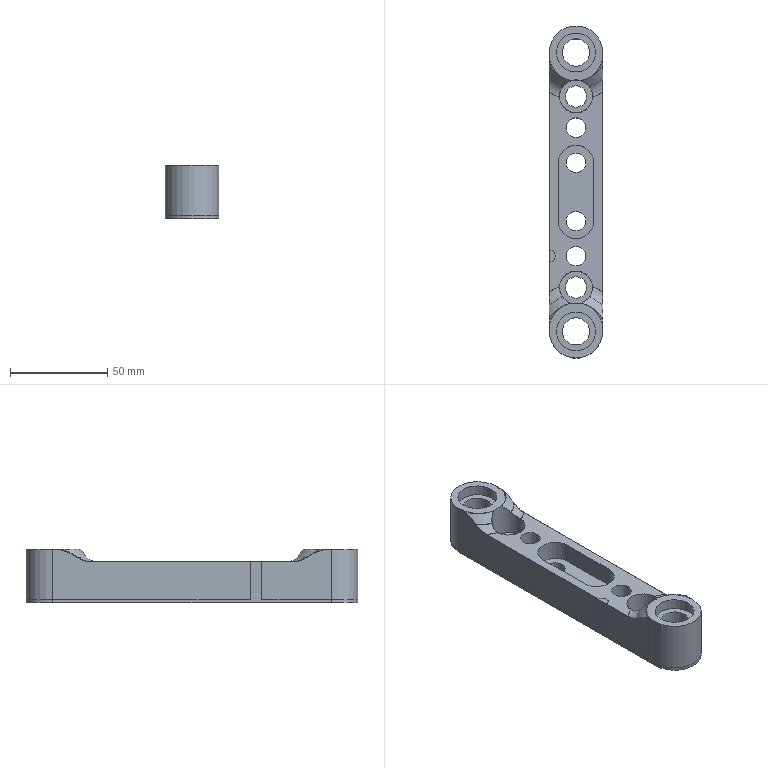NC program | NX | posted with a generic post | part box 27.4 x 170.48 x 27.5 mm
Lines 14728 to 16455 of 16455:
(DRILLING_1 , TOOL : D14钻头)
N29376 T12 M6
N29378 G54
N29380 G17 G0 G90 X-71.54 Y0. B0. C0. S800 M3
N29382 G43 Z30. H12
N29384 G94 G81 G98 Z-28.5 F100. R3.
N29386 X71.54
N29388 G80
N29390 G0 X71.54 Y0. Z30.
N29392 M5
(DRILLING_2 , TOOL : D10镗刀)
N29394 T13 M6
N29396 G54
N29398 G17 G0 G90 X-33. Y0. B0. C0. S800 M3
N29400 G43 Z30. H13
N29402 G94 G86 G98 Z-29.5 F60. R-3.5
N29404 X33.
N29406 G80
N29408 G0 X33. Y0. Z30.
N29410 M5
(DRILLING_3 , TOOL : D20镗刀)
N29412 T14 M6
N29414 G54
N29416 G17 G0 G90 X-71.54 Y0. B0. C0. S800 M3
N29418 G43 Z30. H14
N29420 G94 G86 G98 Z-5.5 F60. R3.
N29422 X71.54
N29424 G80
N29426 G0 X71.54 Y0. Z30.
N29428 M5
(PLANAR_MILL_3_COPY_COPY_COPY_1_COPY , TOOL : D6倒角刀)
N29430 T11 M6
N29432 G54
N29434 G17 G0 G90 X-69.54 Y3.231 B0. C0. S3500 M3
N29436 G43 Z30. H11
N29438 Z-5.8
N29440 G94 G1 Z-7.8 F800.
N29442 Y3.8
N29444 G3 X-71.54 Y5.8 R2.
N29446 X-77.34 Y0. R5.8
N29448 X-71.54 Y5.8 R-5.8
N29450 X-73.54 Y3.8 R2.
N29452 G1 Y3.231
N29454 Z-5.8
N29456 G0 Z30.
N29458 X73.54
N29460 Z-5.8
N29462 G1 Z-7.8
N29464 Y3.8
N29466 G3 X71.54 Y5.8 R2.
N29468 X65.74 Y0. R5.8
N29470 X71.54 Y5.8 R-5.8
N29472 X69.54 Y3.8 R2.
N29474 G1 Y3.231
N29476 Z-5.8
N29478 G0 Z30.
(PLANAR_MILL_3_COPY_COPY_COPY_1_COPY_COPY_1 , TOOL : D6倒角刀)
N29480 X-14. Y1.96
N29482 Z-16.5
N29484 G1 Z-18.5
N29486 Y2.2
N29488 G3 X-15. Y3.2 R1.
N29490 X-18.2 Y0. R3.2
N29492 X-15. Y3.2 R-3.2
N29494 X-16. Y2.2 R1.
N29496 G1 Y1.96
N29498 Z-16.5
N29500 G0 Z30.
N29502 X16.
N29504 Z-16.5
N29506 G1 Z-18.5
N29508 Y2.2
N29510 G3 X15. Y3.2 R1.
N29512 X11.8 Y0. R3.2
N29514 X15. Y3.2 R-3.2
N29516 X14. Y2.2 R1.
N29518 G1 Y1.96
N29520 Z-16.5
N29522 G0 Z30.
N29524 M5
(THREAD_MILLING , TOOL : M16螺纹铣刀)
N29526 T15 M6
N29528 G54
N29530 G17 G0 G90 X-71.54 Y0. B0. C0. S3000 M3
N29532 G43 Z30. H15
N29534 Z-29.182
N29536 G41 G94 G1 X-72.223 Y-1.391 F300. D15
N29538 G3 X-71.54 Y-2.3 Z-29. R0.711
N29540 X-71.54 Y-2.3 Z-27. I0. J2.3
N29542 X-70.857 Y-1.391 Z-26.818 R0.711
N29544 G40
N29546 G1 X-71.54 Y0.
N29548 G0 Z-23.182
N29550 G41 G1 X-72.223 Y-1.391
N29552 G3 X-71.54 Y-2.3 Z-23. R0.711
N29554 X-71.54 Y-2.3 Z-21. I0. J2.3
N29556 X-70.857 Y-1.391 Z-20.818 R0.711
N29558 G40
N29560 G1 X-71.54 Y0.
N29562 G0 Z-17.182
N29564 G41 G1 X-72.223 Y-1.391
N29566 G3 X-71.54 Y-2.3 Z-17. R0.711
N29568 X-71.54 Y-2.3 Z-15. I0. J2.3
N29570 X-70.857 Y-1.391 Z-14.818 R0.711
N29572 G40
N29574 G1 X-71.54 Y0.
N29576 G0 Z-11.182
N29578 G41 G1 X-72.223 Y-1.391
N29580 G3 X-71.54 Y-2.3 Z-11. R0.711
N29582 X-71.54 Y-2.3 Z-9. I0. J2.3
N29584 X-70.857 Y-1.391 Z-8.818 R0.711
N29586 G40
N29588 G1 X-71.54 Y0.
N29590 G0 Z-5.182
N29592 G41 G1 X-72.223 Y-1.391
N29594 G3 X-71.54 Y-2.3 Z-5. R0.711
N29596 X-71.54 Y-2.3 Z-3. I0. J2.3
N29598 X-71.54 Y-2.3 Z-1. I0. J2.3
N29600 X-70.857 Y-1.391 Z-0.818 R0.711
N29602 G40
N29604 G1 X-71.54 Y0.
N29606 G0 Z-29.22
N29608 G41 G1 X-72.371 Y-1.308
N29610 G3 X-71.54 Y-2.55 Z-29. R0.899
N29612 X-71.54 Y-2.55 Z-27. I0. J2.55
N29614 X-70.709 Y-1.308 Z-26.78 R0.899
N29616 G40
N29618 G1 X-71.54 Y0.
N29620 G0 Z-23.22
N29622 G41 G1 X-72.371 Y-1.308
N29624 G3 X-71.54 Y-2.55 Z-23. R0.899
N29626 X-71.54 Y-2.55 Z-21. I0. J2.55
N29628 X-70.709 Y-1.308 Z-20.78 R0.899
N29630 G40
N29632 G1 X-71.54 Y0.
N29634 G0 Z-17.22
N29636 G41 G1 X-72.371 Y-1.308
N29638 G3 X-71.54 Y-2.55 Z-17. R0.899
N29640 X-71.54 Y-2.55 Z-15. I0. J2.55
N29642 X-70.709 Y-1.308 Z-14.78 R0.899
N29644 G40
N29646 G1 X-71.54 Y0.
N29648 G0 Z-11.22
N29650 G41 G1 X-72.371 Y-1.308
N29652 G3 X-71.54 Y-2.55 Z-11. R0.899
N29654 X-71.54 Y-2.55 Z-9. I0. J2.55
N29656 X-70.709 Y-1.308 Z-8.78 R0.899
N29658 G40
N29660 G1 X-71.54 Y0.
N29662 G0 Z-5.22
N29664 G41 G1 X-72.371 Y-1.308
N29666 G3 X-71.54 Y-2.55 Z-5. R0.899
N29668 X-71.54 Y-2.55 Z-3. I0. J2.55
N29670 X-71.54 Y-2.55 Z-1. I0. J2.55
N29672 X-70.709 Y-1.308 Z-0.78 R0.899
N29674 G40
N29676 G1 X-71.54 Y0.
N29678 G0 Z-29.251
N29680 G41 G1 X-72.49 Y-1.225
N29682 G3 X-71.54 Y-2.8 Z-29. R1.074
N29684 X-71.54 Y-2.8 Z-27. I0. J2.8
N29686 X-70.59 Y-1.225 Z-26.749 R1.074
N29688 G40
N29690 G1 X-71.54 Y0.
N29692 G0 Z-23.251
N29694 G41 G1 X-72.49 Y-1.225
N29696 G3 X-71.54 Y-2.8 Z-23. R1.074
N29698 X-71.54 Y-2.8 Z-21. I0. J2.8
N29700 X-70.59 Y-1.225 Z-20.749 R1.074
N29702 G40
N29704 G1 X-71.54 Y0.
N29706 G0 Z-17.251
N29708 G41 G1 X-72.49 Y-1.225
N29710 G3 X-71.54 Y-2.8 Z-17. R1.074
N29712 X-71.54 Y-2.8 Z-15. I0. J2.8
N29714 X-70.59 Y-1.225 Z-14.749 R1.074
N29716 G40
N29718 G1 X-71.54 Y0.
N29720 G0 Z-11.251
N29722 G41 G1 X-72.49 Y-1.225
N29724 G3 X-71.54 Y-2.8 Z-11. R1.074
N29726 X-71.54 Y-2.8 Z-9. I0. J2.8
N29728 X-70.59 Y-1.225 Z-8.749 R1.074
N29730 G40
N29732 G1 X-71.54 Y0.
N29734 G0 Z-5.251
N29736 G41 G1 X-72.49 Y-1.225
N29738 G3 X-71.54 Y-2.8 Z-5. R1.074
N29740 X-71.54 Y-2.8 Z-3. I0. J2.8
N29742 X-71.54 Y-2.8 Z-1. I0. J2.8
N29744 X-70.59 Y-1.225 Z-0.749 R1.074
N29746 G40
N29748 G1 X-71.54 Y0.
N29750 G0 Z-29.277
N29752 G41 G1 X-72.587 Y-1.143
N29754 G3 X-71.54 Y-3.05 Z-29. R1.241
N29756 X-71.54 Y-3.05 Z-27. I0. J3.05
N29758 X-70.493 Y-1.143 Z-26.723 R1.241
N29760 G40
N29762 G1 X-71.54 Y0.
N29764 G0 Z-23.277
N29766 G41 G1 X-72.587 Y-1.143
N29768 G3 X-71.54 Y-3.05 Z-23. R1.241
N29770 X-71.54 Y-3.05 Z-21. I0. J3.05
N29772 X-70.493 Y-1.143 Z-20.723 R1.241
N29774 G40
N29776 G1 X-71.54 Y0.
N29778 G0 Z-17.277
N29780 G41 G1 X-72.587 Y-1.143
N29782 G3 X-71.54 Y-3.05 Z-17. R1.241
N29784 X-71.54 Y-3.05 Z-15. I0. J3.05
N29786 X-70.493 Y-1.143 Z-14.723 R1.241
N29788 G40
N29790 G1 X-71.54 Y0.
N29792 G0 Z-11.277
N29794 G41 G1 X-72.587 Y-1.143
N29796 G3 X-71.54 Y-3.05 Z-11. R1.241
N29798 X-71.54 Y-3.05 Z-9. I0. J3.05
N29800 X-70.493 Y-1.143 Z-8.723 R1.241
N29802 G40
N29804 G1 X-71.54 Y0.
N29806 G0 Z-5.277
N29808 G41 G1 X-72.587 Y-1.143
N29810 G3 X-71.54 Y-3.05 Z-5. R1.241
N29812 X-71.54 Y-3.05 Z-3. I0. J3.05
N29814 X-71.54 Y-3.05 Z-1. I0. J3.05
N29816 X-70.493 Y-1.143 Z-0.723 R1.241
N29818 G40
N29820 G1 X-71.54 Y0.
N29822 G0 Z-29.277
N29824 G41 G1 X-72.587 Y-1.143
N29826 G3 X-71.54 Y-3.05 Z-29. R1.241
N29828 X-71.54 Y-3.05 Z-27. I0. J3.05
N29830 X-70.493 Y-1.143 Z-26.723 R1.241
N29832 G40
N29834 G1 X-71.54 Y0.
N29836 G0 Z-23.277
N29838 G41 G1 X-72.587 Y-1.143
N29840 G3 X-71.54 Y-3.05 Z-23. R1.241
N29842 X-71.54 Y-3.05 Z-21. I0. J3.05
N29844 X-70.493 Y-1.143 Z-20.723 R1.241
N29846 G40
N29848 G1 X-71.54 Y0.
N29850 G0 Z-17.277
N29852 G41 G1 X-72.587 Y-1.143
N29854 G3 X-71.54 Y-3.05 Z-17. R1.241
N29856 X-71.54 Y-3.05 Z-15. I0. J3.05
N29858 X-70.493 Y-1.143 Z-14.723 R1.241
N29860 G40
N29862 G1 X-71.54 Y0.
N29864 G0 Z-11.277
N29866 G41 G1 X-72.587 Y-1.143
N29868 G3 X-71.54 Y-3.05 Z-11. R1.241
N29870 X-71.54 Y-3.05 Z-9. I0. J3.05
N29872 X-70.493 Y-1.143 Z-8.723 R1.241
N29874 G40
N29876 G1 X-71.54 Y0.
N29878 G0 Z-5.277
N29880 G41 G1 X-72.587 Y-1.143
N29882 G3 X-71.54 Y-3.05 Z-5. R1.241
N29884 X-71.54 Y-3.05 Z-3. I0. J3.05
N29886 X-71.54 Y-3.05 Z-1. I0. J3.05
N29888 X-70.493 Y-1.143 Z-0.723 R1.241
N29890 G40
N29892 G1 X-71.54 Y0.
N29894 G0 Z-29.277
N29896 G41 G1 X-72.587 Y-1.143
N29898 G3 X-71.54 Y-3.05 Z-29. R1.241
N29900 X-71.54 Y-3.05 Z-27. I0. J3.05
N29902 X-70.493 Y-1.143 Z-26.723 R1.241
N29904 G40
N29906 G1 X-71.54 Y0.
N29908 G0 Z-23.277
N29910 G41 G1 X-72.587 Y-1.143
N29912 G3 X-71.54 Y-3.05 Z-23. R1.241
N29914 X-71.54 Y-3.05 Z-21. I0. J3.05
N29916 X-70.493 Y-1.143 Z-20.723 R1.241
N29918 G40
N29920 G1 X-71.54 Y0.
N29922 G0 Z-17.277
N29924 G41 G1 X-72.587 Y-1.143
N29926 G3 X-71.54 Y-3.05 Z-17. R1.241
N29928 X-71.54 Y-3.05 Z-15. I0. J3.05
N29930 X-70.493 Y-1.143 Z-14.723 R1.241
N29932 G40
N29934 G1 X-71.54 Y0.
N29936 G0 Z-11.277
N29938 G41 G1 X-72.587 Y-1.143
N29940 G3 X-71.54 Y-3.05 Z-11. R1.241
N29942 X-71.54 Y-3.05 Z-9. I0. J3.05
N29944 X-70.493 Y-1.143 Z-8.723 R1.241
N29946 G40
N29948 G1 X-71.54 Y0.
N29950 G0 Z-5.277
N29952 G41 G1 X-72.587 Y-1.143
N29954 G3 X-71.54 Y-3.05 Z-5. R1.241
N29956 X-71.54 Y-3.05 Z-3. I0. J3.05
N29958 X-71.54 Y-3.05 Z-1. I0. J3.05
N29960 X-70.493 Y-1.143 Z-0.723 R1.241
N29962 G40
N29964 G1 X-71.54 Y0.
N29966 G0 Z30.
N29968 X71.54
N29970 Z-29.182
N29972 G41 G1 X70.857 Y-1.391
N29974 G3 X71.54 Y-2.3 Z-29. R0.711
N29976 X71.54 Y-2.3 Z-27. I0. J2.3
N29978 X72.223 Y-1.391 Z-26.818 R0.711
N29980 G40
N29982 G1 X71.54 Y0.
N29984 G0 Z-23.182
N29986 G41 G1 X70.857 Y-1.391
N29988 G3 X71.54 Y-2.3 Z-23. R0.711
N29990 X71.54 Y-2.3 Z-21. I0. J2.3
N29992 X72.223 Y-1.391 Z-20.818 R0.711
N29994 G40
N29996 G1 X71.54 Y0.
N29998 G0 Z-17.182
N30000 G41 G1 X70.857 Y-1.391
N30002 G3 X71.54 Y-2.3 Z-17. R0.711
N30004 X71.54 Y-2.3 Z-15. I0. J2.3
N30006 X72.223 Y-1.391 Z-14.818 R0.711
N30008 G40
N30010 G1 X71.54 Y0.
N30012 G0 Z-11.182
N30014 G41 G1 X70.857 Y-1.391
N30016 G3 X71.54 Y-2.3 Z-11. R0.711
N30018 X71.54 Y-2.3 Z-9. I0. J2.3
N30020 X72.223 Y-1.391 Z-8.818 R0.711
N30022 G40
N30024 G1 X71.54 Y0.
N30026 G0 Z-5.182
N30028 G41 G1 X70.857 Y-1.391
N30030 G3 X71.54 Y-2.3 Z-5. R0.711
N30032 X71.54 Y-2.3 Z-3. I0. J2.3
N30034 X71.54 Y-2.3 Z-1. I0. J2.3
N30036 X72.223 Y-1.391 Z-0.818 R0.711
N30038 G40
N30040 G1 X71.54 Y0.
N30042 G0 Z-29.22
N30044 G41 G1 X70.709 Y-1.308
N30046 G3 X71.54 Y-2.55 Z-29. R0.899
N30048 X71.54 Y-2.55 Z-27. I0. J2.55
N30050 X72.371 Y-1.308 Z-26.78 R0.899
N30052 G40
N30054 G1 X71.54 Y0.
N30056 G0 Z-23.22
N30058 G41 G1 X70.709 Y-1.308
N30060 G3 X71.54 Y-2.55 Z-23. R0.899
N30062 X71.54 Y-2.55 Z-21. I0. J2.55
N30064 X72.371 Y-1.308 Z-20.78 R0.899
N30066 G40
N30068 G1 X71.54 Y0.
N30070 G0 Z-17.22
N30072 G41 G1 X70.709 Y-1.308
N30074 G3 X71.54 Y-2.55 Z-17. R0.899
N30076 X71.54 Y-2.55 Z-15. I0. J2.55
N30078 X72.371 Y-1.308 Z-14.78 R0.899
N30080 G40
N30082 G1 X71.54 Y0.
N30084 G0 Z-11.22
N30086 G41 G1 X70.709 Y-1.308
N30088 G3 X71.54 Y-2.55 Z-11. R0.899
N30090 X71.54 Y-2.55 Z-9. I0. J2.55
N30092 X72.371 Y-1.308 Z-8.78 R0.899
N30094 G40
N30096 G1 X71.54 Y0.
N30098 G0 Z-5.22
N30100 G41 G1 X70.709 Y-1.308
N30102 G3 X71.54 Y-2.55 Z-5. R0.899
N30104 X71.54 Y-2.55 Z-3. I0. J2.55
N30106 X71.54 Y-2.55 Z-1. I0. J2.55
N30108 X72.371 Y-1.308 Z-0.78 R0.899
N30110 G40
N30112 G1 X71.54 Y0.
N30114 G0 Z-29.251
N30116 G41 G1 X70.59 Y-1.225
N30118 G3 X71.54 Y-2.8 Z-29. R1.074
N30120 X71.54 Y-2.8 Z-27. I0. J2.8
N30122 X72.49 Y-1.225 Z-26.749 R1.074
N30124 G40
N30126 G1 X71.54 Y0.
N30128 G0 Z-23.251
N30130 G41 G1 X70.59 Y-1.225
N30132 G3 X71.54 Y-2.8 Z-23. R1.074
N30134 X71.54 Y-2.8 Z-21. I0. J2.8
N30136 X72.49 Y-1.225 Z-20.749 R1.074
N30138 G40
N30140 G1 X71.54 Y0.
N30142 G0 Z-17.251
N30144 G41 G1 X70.59 Y-1.225
N30146 G3 X71.54 Y-2.8 Z-17. R1.074
N30148 X71.54 Y-2.8 Z-15. I0. J2.8
N30150 X72.49 Y-1.225 Z-14.749 R1.074
N30152 G40
N30154 G1 X71.54 Y0.
N30156 G0 Z-11.251
N30158 G41 G1 X70.59 Y-1.225
N30160 G3 X71.54 Y-2.8 Z-11. R1.074
N30162 X71.54 Y-2.8 Z-9. I0. J2.8
N30164 X72.49 Y-1.225 Z-8.749 R1.074
N30166 G40
N30168 G1 X71.54 Y0.
N30170 G0 Z-5.251
N30172 G41 G1 X70.59 Y-1.225
N30174 G3 X71.54 Y-2.8 Z-5. R1.074
N30176 X71.54 Y-2.8 Z-3. I0. J2.8
N30178 X71.54 Y-2.8 Z-1. I0. J2.8
N30180 X72.49 Y-1.225 Z-0.749 R1.074
N30182 G40
N30184 G1 X71.54 Y0.
N30186 G0 Z-29.277
N30188 G41 G1 X70.493 Y-1.143
N30190 G3 X71.54 Y-3.05 Z-29. R1.241
N30192 X71.54 Y-3.05 Z-27. I0. J3.05
N30194 X72.587 Y-1.143 Z-26.723 R1.241
N30196 G40
N30198 G1 X71.54 Y0.
N30200 G0 Z-23.277
N30202 G41 G1 X70.493 Y-1.143
N30204 G3 X71.54 Y-3.05 Z-23. R1.241
N30206 X71.54 Y-3.05 Z-21. I0. J3.05
N30208 X72.587 Y-1.143 Z-20.723 R1.241
N30210 G40
N30212 G1 X71.54 Y0.
N30214 G0 Z-17.277
N30216 G41 G1 X70.493 Y-1.143
N30218 G3 X71.54 Y-3.05 Z-17. R1.241
N30220 X71.54 Y-3.05 Z-15. I0. J3.05
N30222 X72.587 Y-1.143 Z-14.723 R1.241
N30224 G40
N30226 G1 X71.54 Y0.
N30228 G0 Z-11.277
N30230 G41 G1 X70.493 Y-1.143
N30232 G3 X71.54 Y-3.05 Z-11. R1.241
N30234 X71.54 Y-3.05 Z-9. I0. J3.05
N30236 X72.587 Y-1.143 Z-8.723 R1.241
N30238 G40
N30240 G1 X71.54 Y0.
N30242 G0 Z-5.277
N30244 G41 G1 X70.493 Y-1.143
N30246 G3 X71.54 Y-3.05 Z-5. R1.241
N30248 X71.54 Y-3.05 Z-3. I0. J3.05
N30250 X71.54 Y-3.05 Z-1. I0. J3.05
N30252 X72.587 Y-1.143 Z-0.723 R1.241
N30254 G40
N30256 G1 X71.54 Y0.
N30258 G0 Z-29.277
N30260 G41 G1 X70.493 Y-1.143
N30262 G3 X71.54 Y-3.05 Z-29. R1.241
N30264 X71.54 Y-3.05 Z-27. I0. J3.05
N30266 X72.587 Y-1.143 Z-26.723 R1.241
N30268 G40
N30270 G1 X71.54 Y0.
N30272 G0 Z-23.277
N30274 G41 G1 X70.493 Y-1.143
N30276 G3 X71.54 Y-3.05 Z-23. R1.241
N30278 X71.54 Y-3.05 Z-21. I0. J3.05
N30280 X72.587 Y-1.143 Z-20.723 R1.241
N30282 G40
N30284 G1 X71.54 Y0.
N30286 G0 Z-17.277
N30288 G41 G1 X70.493 Y-1.143
N30290 G3 X71.54 Y-3.05 Z-17. R1.241
N30292 X71.54 Y-3.05 Z-15. I0. J3.05
N30294 X72.587 Y-1.143 Z-14.723 R1.241
N30296 G40
N30298 G1 X71.54 Y0.
N30300 G0 Z-11.277
N30302 G41 G1 X70.493 Y-1.143
N30304 G3 X71.54 Y-3.05 Z-11. R1.241
N30306 X71.54 Y-3.05 Z-9. I0. J3.05
N30308 X72.587 Y-1.143 Z-8.723 R1.241
N30310 G40
N30312 G1 X71.54 Y0.
N30314 G0 Z-5.277
N30316 G41 G1 X70.493 Y-1.143
N30318 G3 X71.54 Y-3.05 Z-5. R1.241
N30320 X71.54 Y-3.05 Z-3. I0. J3.05
N30322 X71.54 Y-3.05 Z-1. I0. J3.05
N30324 X72.587 Y-1.143 Z-0.723 R1.241
N30326 G40
N30328 G1 X71.54 Y0.
N30330 G0 Z-29.277
N30332 G41 G1 X70.493 Y-1.143
N30334 G3 X71.54 Y-3.05 Z-29. R1.241
N30336 X71.54 Y-3.05 Z-27. I0. J3.05
N30338 X72.587 Y-1.143 Z-26.723 R1.241
N30340 G40
N30342 G1 X71.54 Y0.
N30344 G0 Z-23.277
N30346 G41 G1 X70.493 Y-1.143
N30348 G3 X71.54 Y-3.05 Z-23. R1.241
N30350 X71.54 Y-3.05 Z-21. I0. J3.05
N30352 X72.587 Y-1.143 Z-20.723 R1.241
N30354 G40
N30356 G1 X71.54 Y0.
N30358 G0 Z-17.277
N30360 G41 G1 X70.493 Y-1.143
N30362 G3 X71.54 Y-3.05 Z-17. R1.241
N30364 X71.54 Y-3.05 Z-15. I0. J3.05
N30366 X72.587 Y-1.143 Z-14.723 R1.241
N30368 G40
N30370 G1 X71.54 Y0.
N30372 G0 Z-11.277
N30374 G41 G1 X70.493 Y-1.143
N30376 G3 X71.54 Y-3.05 Z-11. R1.241
N30378 X71.54 Y-3.05 Z-9. I0. J3.05
N30380 X72.587 Y-1.143 Z-8.723 R1.241
N30382 G40
N30384 G1 X71.54 Y0.
N30386 G0 Z-5.277
N30388 G41 G1 X70.493 Y-1.143
N30390 G3 X71.54 Y-3.05 Z-5. R1.241
N30392 X71.54 Y-3.05 Z-3. I0. J3.05
N30394 X71.54 Y-3.05 Z-1. I0. J3.05
N30396 X72.587 Y-1.143 Z-0.723 R1.241
N30398 G40
N30400 G1 X71.54 Y0.
N30402 G0 Z30.
N30404 M5
(PLANAR_MILL_14 , TOOL : D5开粗)
N30406 T20 M6
N30408 G54
N30410 G17 G0 G90 X33.305 Y-17.397 B0. C0. S3500 M3
N30412 G43 Z30. H20
N30414 Z-4.699
N30416 G94 G1 Z-6.699 F600.
N30418 G41 X33.34 Y-17.2 D20
N30420 Y-13.7
N30422 G3 X32.84 Y-13.2 R0.5
N30424 X32.34 Y-13.7 R0.5
N30426 G1 Y-17.2
N30428 G40
N30430 X32.375 Y-17.397
N30432 Z-4.699
N30434 G0 X33.305 Z-4.898
N30436 G1 Z-6.898
N30438 G41 X33.34 Y-17.2
N30440 Y-13.7
N30442 G3 X32.84 Y-13.2 R0.5
N30444 X32.34 Y-13.7 R0.5
N30446 G1 Y-17.2
N30448 G40
N30450 X32.375 Y-17.397
N30452 Z-4.898
N30454 G0 X33.305 Z-5.097
N30456 G1 Z-7.097
N30458 G41 X33.34 Y-17.2
N30460 Y-13.7
N30462 G3 X32.84 Y-13.2 R0.5
N30464 X32.34 Y-13.7 R0.5
N30466 G1 Y-17.2
N30468 G40
N30470 X32.375 Y-17.397
N30472 Z-5.097
N30474 G0 X33.305 Z-5.296
N30476 G1 Z-7.296
N30478 G41 X33.34 Y-17.2
N30480 Y-13.7
N30482 G3 X32.84 Y-13.2 R0.5
N30484 X32.34 Y-13.7 R0.5
N30486 G1 Y-17.2
N30488 G40
N30490 X32.375 Y-17.397
N30492 Z-5.296
N30494 G0 X33.305 Z-5.495
N30496 G1 Z-7.495
N30498 G41 X33.34 Y-17.2
N30500 Y-13.7
N30502 G3 X32.84 Y-13.2 R0.5
N30504 X32.34 Y-13.7 R0.5
N30506 G1 Y-17.2
N30508 G40
N30510 X32.375 Y-17.397
N30512 Z-5.495
N30514 G0 X33.305 Z-5.694
N30516 G1 Z-7.694
N30518 G41 X33.34 Y-17.2
N30520 Y-13.7
N30522 G3 X32.84 Y-13.2 R0.5
N30524 X32.34 Y-13.7 R0.5
N30526 G1 Y-17.2
N30528 G40
N30530 X32.375 Y-17.397
N30532 Z-5.694
N30534 G0 X33.305 Z-5.894
N30536 G1 Z-7.894
N30538 G41 X33.34 Y-17.2
N30540 Y-13.7
N30542 G3 X32.84 Y-13.2 R0.5
N30544 X32.34 Y-13.7 R0.5
N30546 G1 Y-17.2
N30548 G40
N30550 X32.375 Y-17.397
N30552 Z-5.894
N30554 G0 X33.305 Z-6.093
N30556 G1 Z-8.093
N30558 G41 X33.34 Y-17.2
N30560 Y-13.7
N30562 G3 X32.84 Y-13.2 R0.5
N30564 X32.34 Y-13.7 R0.5
N30566 G1 Y-17.2
N30568 G40
N30570 X32.375 Y-17.397
N30572 Z-6.093
N30574 G0 X33.305 Z-6.292
N30576 G1 Z-8.292
N30578 G41 X33.34 Y-17.2
N30580 Y-13.7
N30582 G3 X32.84 Y-13.2 R0.5
N30584 X32.34 Y-13.7 R0.5
N30586 G1 Y-17.2
N30588 G40
N30590 X32.375 Y-17.397
N30592 Z-6.292
N30594 G0 X33.305 Z-6.491
N30596 G1 Z-8.491
N30598 G41 X33.34 Y-17.2
N30600 Y-13.7
N30602 G3 X32.84 Y-13.2 R0.5
N30604 X32.34 Y-13.7 R0.5
N30606 G1 Y-17.2
N30608 G40
N30610 X32.375 Y-17.397
N30612 Z-6.491
N30614 G0 X33.305 Z-6.69
N30616 G1 Z-8.69
N30618 G41 X33.34 Y-17.2
N30620 Y-13.7
N30622 G3 X32.84 Y-13.2 R0.5
N30624 X32.34 Y-13.7 R0.5
N30626 G1 Y-17.2
N30628 G40
N30630 X32.375 Y-17.397
N30632 Z-6.69
N30634 G0 X33.305 Z-6.889
N30636 G1 Z-8.889
N30638 G41 X33.34 Y-17.2
N30640 Y-13.7
N30642 G3 X32.84 Y-13.2 R0.5
N30644 X32.34 Y-13.7 R0.5
N30646 G1 Y-17.2
N30648 G40
N30650 X32.375 Y-17.397
N30652 Z-6.889
N30654 G0 X33.305 Z-7.088
N30656 G1 Z-9.088
N30658 G41 X33.34 Y-17.2
N30660 Y-13.7
N30662 G3 X32.84 Y-13.2 R0.5
N30664 X32.34 Y-13.7 R0.5
N30666 G1 Y-17.2
N30668 G40
N30670 X32.375 Y-17.397
N30672 Z-7.088
N30674 G0 X33.305 Z-7.287
N30676 G1 Z-9.287
N30678 G41 X33.34 Y-17.2
N30680 Y-13.7
N30682 G3 X32.84 Y-13.2 R0.5
N30684 X32.34 Y-13.7 R0.5
N30686 G1 Y-17.2
N30688 G40
N30690 X32.375 Y-17.397
N30692 Z-7.287
N30694 G0 X33.305 Z-7.486
N30696 G1 Z-9.486
N30698 G41 X33.34 Y-17.2
N30700 Y-13.7
N30702 G3 X32.84 Y-13.2 R0.5
N30704 X32.34 Y-13.7 R0.5
N30706 G1 Y-17.2
N30708 G40
N30710 X32.375 Y-17.397
N30712 Z-7.486
N30714 G0 X33.305 Z-7.685
N30716 G1 Z-9.685
N30718 G41 X33.34 Y-17.2
N30720 Y-13.7
N30722 G3 X32.84 Y-13.2 R0.5
N30724 X32.34 Y-13.7 R0.5
N30726 G1 Y-17.2
N30728 G40
N30730 X32.375 Y-17.397
N30732 Z-7.685
N30734 G0 X33.305 Z-7.884
N30736 G1 Z-9.884
N30738 G41 X33.34 Y-17.2
N30740 Y-13.7
N30742 G3 X32.84 Y-13.2 R0.5
N30744 X32.34 Y-13.7 R0.5
N30746 G1 Y-17.2
N30748 G40
N30750 X32.375 Y-17.397
N30752 Z-7.884
N30754 G0 X33.305 Z-8.083
N30756 G1 Z-10.083
N30758 G41 X33.34 Y-17.2
N30760 Y-13.7
N30762 G3 X32.84 Y-13.2 R0.5
N30764 X32.34 Y-13.7 R0.5
N30766 G1 Y-17.2
N30768 G40
N30770 X32.375 Y-17.397
N30772 Z-8.083
N30774 G0 X33.305 Z-8.282
N30776 G1 Z-10.282
N30778 G41 X33.34 Y-17.2
N30780 Y-13.7
N30782 G3 X32.84 Y-13.2 R0.5
N30784 X32.34 Y-13.7 R0.5
N30786 G1 Y-17.2
N30788 G40
N30790 X32.375 Y-17.397
N30792 Z-8.282
N30794 G0 X33.305 Z-8.481
N30796 G1 Z-10.481
N30798 G41 X33.34 Y-17.2
N30800 Y-13.7
N30802 G3 X32.84 Y-13.2 R0.5
N30804 X32.34 Y-13.7 R0.5
N30806 G1 Y-17.2
N30808 G40
N30810 X32.375 Y-17.397
N30812 Z-8.481
N30814 G0 X33.305 Z-8.681
N30816 G1 Z-10.681
N30818 G41 X33.34 Y-17.2
N30820 Y-13.7
N30822 G3 X32.84 Y-13.2 R0.5
N30824 X32.34 Y-13.7 R0.5
N30826 G1 Y-17.2
N30828 G40
N30830 X32.375 Y-17.397
N30832 Z-8.681
N30834 G0 X33.305 Z-8.88
N30836 G1 Z-10.88
N30838 G41 X33.34 Y-17.2
N30840 Y-13.7
N30842 G3 X32.84 Y-13.2 R0.5
N30844 X32.34 Y-13.7 R0.5
N30846 G1 Y-17.2
N30848 G40
N30850 X32.375 Y-17.397
N30852 Z-8.88
N30854 G0 X33.305 Z-9.079
N30856 G1 Z-11.079
N30858 G41 X33.34 Y-17.2
N30860 Y-13.7
N30862 G3 X32.84 Y-13.2 R0.5
N30864 X32.34 Y-13.7 R0.5
N30866 G1 Y-17.2
N30868 G40
N30870 X32.375 Y-17.397
N30872 Z-9.079
N30874 G0 X33.305 Z-9.278
N30876 G1 Z-11.278
N30878 G41 X33.34 Y-17.2
N30880 Y-13.7
N30882 G3 X32.84 Y-13.2 R0.5
N30884 X32.34 Y-13.7 R0.5
N30886 G1 Y-17.2
N30888 G40
N30890 X32.375 Y-17.397
N30892 Z-9.278
N30894 G0 X33.305 Z-9.477
N30896 G1 Z-11.477
N30898 G41 X33.34 Y-17.2
N30900 Y-13.7
N30902 G3 X32.84 Y-13.2 R0.5
N30904 X32.34 Y-13.7 R0.5
N30906 G1 Y-17.2
N30908 G40
N30910 X32.375 Y-17.397
N30912 Z-9.477
N30914 G0 X33.305 Z-9.676
N30916 G1 Z-11.676
N30918 G41 X33.34 Y-17.2
N30920 Y-13.7
N30922 G3 X32.84 Y-13.2 R0.5
N30924 X32.34 Y-13.7 R0.5
N30926 G1 Y-17.2
N30928 G40
N30930 X32.375 Y-17.397
N30932 Z-9.676
N30934 G0 X33.305 Z-9.875
N30936 G1 Z-11.875
N30938 G41 X33.34 Y-17.2
N30940 Y-13.7
N30942 G3 X32.84 Y-13.2 R0.5
N30944 X32.34 Y-13.7 R0.5
N30946 G1 Y-17.2
N30948 G40
N30950 X32.375 Y-17.397
N30952 Z-9.875
N30954 G0 X33.305 Z-10.074
N30956 G1 Z-12.074
N30958 G41 X33.34 Y-17.2
N30960 Y-13.7
N30962 G3 X32.84 Y-13.2 R0.5
N30964 X32.34 Y-13.7 R0.5
N30966 G1 Y-17.2
N30968 G40
N30970 X32.375 Y-17.397
N30972 Z-10.074
N30974 G0 X33.305 Z-10.273
N30976 G1 Z-12.273
N30978 G41 X33.34 Y-17.2
N30980 Y-13.7
N30982 G3 X32.84 Y-13.2 R0.5
N30984 X32.34 Y-13.7 R0.5
N30986 G1 Y-17.2
N30988 G40
N30990 X32.375 Y-17.397
N30992 Z-10.273
N30994 G0 X33.305 Z-10.472
N30996 G1 Z-12.472
N30998 G41 X33.34 Y-17.2
N31000 Y-13.7
N31002 G3 X32.84 Y-13.2 R0.5
N31004 X32.34 Y-13.7 R0.5
N31006 G1 Y-17.2
N31008 G40
N31010 X32.375 Y-17.397
N31012 Z-10.472
N31014 G0 X33.305 Z-10.671
N31016 G1 Z-12.671
N31018 G41 X33.34 Y-17.2
N31020 Y-13.7
N31022 G3 X32.84 Y-13.2 R0.5
N31024 X32.34 Y-13.7 R0.5
N31026 G1 Y-17.2
N31028 G40
N31030 X32.375 Y-17.397
N31032 Z-10.671
N31034 G0 X33.305 Z-10.87
N31036 G1 Z-12.87
N31038 G41 X33.34 Y-17.2
N31040 Y-13.7
N31042 G3 X32.84 Y-13.2 R0.5
N31044 X32.34 Y-13.7 R0.5
N31046 G1 Y-17.2
N31048 G40
N31050 X32.375 Y-17.397
N31052 Z-10.87
N31054 G0 X33.305 Z-11.069
N31056 G1 Z-13.069
N31058 G41 X33.34 Y-17.2
N31060 Y-13.7
N31062 G3 X32.84 Y-13.2 R0.5
N31064 X32.34 Y-13.7 R0.5
N31066 G1 Y-17.2
N31068 G40
N31070 X32.375 Y-17.397
N31072 Z-11.069
N31074 G0 X33.305 Z-11.269
N31076 G1 Z-13.269
N31078 G41 X33.34 Y-17.2
N31080 Y-13.7
N31082 G3 X32.84 Y-13.2 R0.5
N31084 X32.34 Y-13.7 R0.5
N31086 G1 Y-17.2
N31088 G40
N31090 X32.375 Y-17.397
N31092 Z-11.269
N31094 G0 X33.305 Z-11.468
N31096 G1 Z-13.468
N31098 G41 X33.34 Y-17.2
N31100 Y-13.7
N31102 G3 X32.84 Y-13.2 R0.5
N31104 X32.34 Y-13.7 R0.5
N31106 G1 Y-17.2
N31108 G40
N31110 X32.375 Y-17.397
N31112 Z-11.468
N31114 G0 X33.305 Z-11.667
N31116 G1 Z-13.667
N31118 G41 X33.34 Y-17.2
N31120 Y-13.7
N31122 G3 X32.84 Y-13.2 R0.5
N31124 X32.34 Y-13.7 R0.5
N31126 G1 Y-17.2
N31128 G40
N31130 X32.375 Y-17.397
N31132 Z-11.667
N31134 G0 X33.305 Z-11.866
N31136 G1 Z-13.866
N31138 G41 X33.34 Y-17.2
N31140 Y-13.7
N31142 G3 X32.84 Y-13.2 R0.5
N31144 X32.34 Y-13.7 R0.5
N31146 G1 Y-17.2
N31148 G40
N31150 X32.375 Y-17.397
N31152 Z-11.866
N31154 G0 X33.305 Z-12.065
N31156 G1 Z-14.065
N31158 G41 X33.34 Y-17.2
N31160 Y-13.7
N31162 G3 X32.84 Y-13.2 R0.5
N31164 X32.34 Y-13.7 R0.5
N31166 G1 Y-17.2
N31168 G40
N31170 X32.375 Y-17.397
N31172 Z-12.065
N31174 G0 X33.305 Z-12.264
N31176 G1 Z-14.264
N31178 G41 X33.34 Y-17.2
N31180 Y-13.7
N31182 G3 X32.84 Y-13.2 R0.5
N31184 X32.34 Y-13.7 R0.5
N31186 G1 Y-17.2
N31188 G40
N31190 X32.375 Y-17.397
N31192 Z-12.264
N31194 G0 X33.305 Z-12.463
N31196 G1 Z-14.463
N31198 G41 X33.34 Y-17.2
N31200 Y-13.7
N31202 G3 X32.84 Y-13.2 R0.5
N31204 X32.34 Y-13.7 R0.5
N31206 G1 Y-17.2
N31208 G40
N31210 X32.375 Y-17.397
N31212 Z-12.463
N31214 G0 X33.305 Z-12.662
N31216 G1 Z-14.662
N31218 G41 X33.34 Y-17.2
N31220 Y-13.7
N31222 G3 X32.84 Y-13.2 R0.5
N31224 X32.34 Y-13.7 R0.5
N31226 G1 Y-17.2
N31228 G40
N31230 X32.375 Y-17.397
N31232 Z-12.662
N31234 G0 X33.305 Z-12.861
N31236 G1 Z-14.861
N31238 G41 X33.34 Y-17.2
N31240 Y-13.7
N31242 G3 X32.84 Y-13.2 R0.5
N31244 X32.34 Y-13.7 R0.5
N31246 G1 Y-17.2
N31248 G40
N31250 X32.375 Y-17.397
N31252 Z-12.861
N31254 G0 X33.305 Z-13.06
N31256 G1 Z-15.06
N31258 G41 X33.34 Y-17.2
N31260 Y-13.7
N31262 G3 X32.84 Y-13.2 R0.5
N31264 X32.34 Y-13.7 R0.5
N31266 G1 Y-17.2
N31268 G40
N31270 X32.375 Y-17.397
N31272 Z-13.06
N31274 G0 X33.305 Z-13.259
N31276 G1 Z-15.259
N31278 G41 X33.34 Y-17.2
N31280 Y-13.7
N31282 G3 X32.84 Y-13.2 R0.5
N31284 X32.34 Y-13.7 R0.5
N31286 G1 Y-17.2
N31288 G40
N31290 X32.375 Y-17.397
N31292 Z-13.259
N31294 G0 X33.305 Z-13.458
N31296 G1 Z-15.458
N31298 G41 X33.34 Y-17.2
N31300 Y-13.7
N31302 G3 X32.84 Y-13.2 R0.5
N31304 X32.34 Y-13.7 R0.5
N31306 G1 Y-17.2
N31308 G40
N31310 X32.375 Y-17.397
N31312 Z-13.458
N31314 G0 X33.305 Z-13.657
N31316 G1 Z-15.657
N31318 G41 X33.34 Y-17.2
N31320 Y-13.7
N31322 G3 X32.84 Y-13.2 R0.5
N31324 X32.34 Y-13.7 R0.5
N31326 G1 Y-17.2
N31328 G40
N31330 X32.375 Y-17.397
N31332 Z-13.657
N31334 G0 X33.305 Z-13.856
N31336 G1 Z-15.856
N31338 G41 X33.34 Y-17.2
N31340 Y-13.7
N31342 G3 X32.84 Y-13.2 R0.5
N31344 X32.34 Y-13.7 R0.5
N31346 G1 Y-17.2
N31348 G40
N31350 X32.375 Y-17.397
N31352 Z-13.856
N31354 G0 X33.305 Z-14.056
N31356 G1 Z-16.056
N31358 G41 X33.34 Y-17.2
N31360 Y-13.7
N31362 G3 X32.84 Y-13.2 R0.5
N31364 X32.34 Y-13.7 R0.5
N31366 G1 Y-17.2
N31368 G40
N31370 X32.375 Y-17.397
N31372 Z-14.056
N31374 G0 X33.305 Z-14.255
N31376 G1 Z-16.255
N31378 G41 X33.34 Y-17.2
N31380 Y-13.7
N31382 G3 X32.84 Y-13.2 R0.5
N31384 X32.34 Y-13.7 R0.5
N31386 G1 Y-17.2
N31388 G40
N31390 X32.375 Y-17.397
N31392 Z-14.255
N31394 G0 X33.305 Z-14.454
N31396 G1 Z-16.454
N31398 G41 X33.34 Y-17.2
N31400 Y-13.7
N31402 G3 X32.84 Y-13.2 R0.5
N31404 X32.34 Y-13.7 R0.5
N31406 G1 Y-17.2
N31408 G40
N31410 X32.375 Y-17.397
N31412 Z-14.454
N31414 G0 X33.305 Z-14.653
N31416 G1 Z-16.653
N31418 G41 X33.34 Y-17.2
N31420 Y-13.7
N31422 G3 X32.84 Y-13.2 R0.5
N31424 X32.34 Y-13.7 R0.5
N31426 G1 Y-17.2
N31428 G40
N31430 X32.375 Y-17.397
N31432 Z-14.653
N31434 G0 X33.305 Z-14.852
N31436 G1 Z-16.852
N31438 G41 X33.34 Y-17.2
N31440 Y-13.7
N31442 G3 X32.84 Y-13.2 R0.5
N31444 X32.34 Y-13.7 R0.5
N31446 G1 Y-17.2
N31448 G40
N31450 X32.375 Y-17.397
N31452 Z-14.852
N31454 G0 X33.305 Z-15.051
N31456 G1 Z-17.051
N31458 G41 X33.34 Y-17.2
N31460 Y-13.7
N31462 G3 X32.84 Y-13.2 R0.5
N31464 X32.34 Y-13.7 R0.5
N31466 G1 Y-17.2
N31468 G40
N31470 X32.375 Y-17.397
N31472 Z-15.051
N31474 G0 X33.305 Z-15.25
N31476 G1 Z-17.25
N31478 G41 X33.34 Y-17.2
N31480 Y-13.7
N31482 G3 X32.84 Y-13.2 R0.5
N31484 X32.34 Y-13.7 R0.5
N31486 G1 Y-17.2
N31488 G40
N31490 X32.375 Y-17.397
N31492 Z-15.25
N31494 G0 X33.305 Z-15.449
N31496 G1 Z-17.449
N31498 G41 X33.34 Y-17.2
N31500 Y-13.7
N31502 G3 X32.84 Y-13.2 R0.5
N31504 X32.34 Y-13.7 R0.5
N31506 G1 Y-17.2
N31508 G40
N31510 X32.375 Y-17.397
N31512 Z-15.449
N31514 G0 X33.305 Z-15.648
N31516 G1 Z-17.648
N31518 G41 X33.34 Y-17.2
N31520 Y-13.7
N31522 G3 X32.84 Y-13.2 R0.5
N31524 X32.34 Y-13.7 R0.5
N31526 G1 Y-17.2
N31528 G40
N31530 X32.375 Y-17.397
N31532 Z-15.648
N31534 G0 X33.305 Z-15.847
N31536 G1 Z-17.847
N31538 G41 X33.34 Y-17.2
N31540 Y-13.7
N31542 G3 X32.84 Y-13.2 R0.5
N31544 X32.34 Y-13.7 R0.5
N31546 G1 Y-17.2
N31548 G40
N31550 X32.375 Y-17.397
N31552 Z-15.847
N31554 G0 X33.305 Z-16.046
N31556 G1 Z-18.046
N31558 G41 X33.34 Y-17.2
N31560 Y-13.7
N31562 G3 X32.84 Y-13.2 R0.5
N31564 X32.34 Y-13.7 R0.5
N31566 G1 Y-17.2
N31568 G40
N31570 X32.375 Y-17.397
N31572 Z-16.046
N31574 G0 X33.305 Z-16.245
N31576 G1 Z-18.245
N31578 G41 X33.34 Y-17.2
N31580 Y-13.7
N31582 G3 X32.84 Y-13.2 R0.5
N31584 X32.34 Y-13.7 R0.5
N31586 G1 Y-17.2
N31588 G40
N31590 X32.375 Y-17.397
N31592 Z-16.245
N31594 G0 X33.305 Z-16.444
N31596 G1 Z-18.444
N31598 G41 X33.34 Y-17.2
N31600 Y-13.7
N31602 G3 X32.84 Y-13.2 R0.5
N31604 X32.34 Y-13.7 R0.5
N31606 G1 Y-17.2
N31608 G40
N31610 X32.375 Y-17.397
N31612 Z-16.444
N31614 G0 X33.305 Z-16.644
N31616 G1 Z-18.644
N31618 G41 X33.34 Y-17.2
N31620 Y-13.7
N31622 G3 X32.84 Y-13.2 R0.5
N31624 X32.34 Y-13.7 R0.5
N31626 G1 Y-17.2
N31628 G40
N31630 X32.375 Y-17.397
N31632 Z-16.644
N31634 G0 X33.305 Z-16.843
N31636 G1 Z-18.843
N31638 G41 X33.34 Y-17.2
N31640 Y-13.7
N31642 G3 X32.84 Y-13.2 R0.5
N31644 X32.34 Y-13.7 R0.5
N31646 G1 Y-17.2
N31648 G40
N31650 X32.375 Y-17.397
N31652 Z-16.843
N31654 G0 X33.305 Z-17.042
N31656 G1 Z-19.042
N31658 G41 X33.34 Y-17.2
N31660 Y-13.7
N31662 G3 X32.84 Y-13.2 R0.5
N31664 X32.34 Y-13.7 R0.5
N31666 G1 Y-17.2
N31668 G40
N31670 X32.375 Y-17.397
N31672 Z-17.042
N31674 G0 X33.305 Z-17.241
N31676 G1 Z-19.241
N31678 G41 X33.34 Y-17.2
N31680 Y-13.7
N31682 G3 X32.84 Y-13.2 R0.5
N31684 X32.34 Y-13.7 R0.5
N31686 G1 Y-17.2
N31688 G40
N31690 X32.375 Y-17.397
N31692 Z-17.241
N31694 G0 X33.305 Z-17.44
N31696 G1 Z-19.44
N31698 G41 X33.34 Y-17.2
N31700 Y-13.7
N31702 G3 X32.84 Y-13.2 R0.5
N31704 X32.34 Y-13.7 R0.5
N31706 G1 Y-17.2
N31708 G40
N31710 X32.375 Y-17.397
N31712 Z-17.44
N31714 G0 X33.305 Z-17.639
N31716 G1 Z-19.639
N31718 G41 X33.34 Y-17.2
N31720 Y-13.7
N31722 G3 X32.84 Y-13.2 R0.5
N31724 X32.34 Y-13.7 R0.5
N31726 G1 Y-17.2
N31728 G40
N31730 X32.375 Y-17.397
N31732 Z-17.639
N31734 G0 X33.305 Z-17.838
N31736 G1 Z-19.838
N31738 G41 X33.34 Y-17.2
N31740 Y-13.7
N31742 G3 X32.84 Y-13.2 R0.5
N31744 X32.34 Y-13.7 R0.5
N31746 G1 Y-17.2
N31748 G40
N31750 X32.375 Y-17.397
N31752 Z-17.838
N31754 G0 X33.305 Z-18.037
N31756 G1 Z-20.037
N31758 G41 X33.34 Y-17.2
N31760 Y-13.7
N31762 G3 X32.84 Y-13.2 R0.5
N31764 X32.34 Y-13.7 R0.5
N31766 G1 Y-17.2
N31768 G40
N31770 X32.375 Y-17.397
N31772 Z-18.037
N31774 G0 X33.305 Z-18.236
N31776 G1 Z-20.236
N31778 G41 X33.34 Y-17.2
N31780 Y-13.7
N31782 G3 X32.84 Y-13.2 R0.5
N31784 X32.34 Y-13.7 R0.5
N31786 G1 Y-17.2
N31788 G40
N31790 X32.375 Y-17.397
N31792 Z-18.236
N31794 G0 X33.305 Z-18.435
N31796 G1 Z-20.435
N31798 G41 X33.34 Y-17.2
N31800 Y-13.7
N31802 G3 X32.84 Y-13.2 R0.5
N31804 X32.34 Y-13.7 R0.5
N31806 G1 Y-17.2
N31808 G40
N31810 X32.375 Y-17.397
N31812 Z-18.435
N31814 G0 X33.305 Z-18.634
N31816 G1 Z-20.634
N31818 G41 X33.34 Y-17.2
N31820 Y-13.7
N31822 G3 X32.84 Y-13.2 R0.5
N31824 X32.34 Y-13.7 R0.5
N31826 G1 Y-17.2
N31828 G40
N31830 X32.375 Y-17.397
N31832 Z-18.634
N31834 G0 X33.305 Z-18.833
N31836 G1 Z-20.833
N31838 G41 X33.34 Y-17.2
N31840 Y-13.7
N31842 G3 X32.84 Y-13.2 R0.5
N31844 X32.34 Y-13.7 R0.5
N31846 G1 Y-17.2
N31848 G40
N31850 X32.375 Y-17.397
N31852 Z-18.833
N31854 G0 X33.305 Z-19.032
N31856 G1 Z-21.032
N31858 G41 X33.34 Y-17.2
N31860 Y-13.7
N31862 G3 X32.84 Y-13.2 R0.5
N31864 X32.34 Y-13.7 R0.5
N31866 G1 Y-17.2
N31868 G40
N31870 X32.375 Y-17.397
N31872 Z-19.032
N31874 G0 X33.305 Z-19.231
N31876 G1 Z-21.231
N31878 G41 X33.34 Y-17.2
N31880 Y-13.7
N31882 G3 X32.84 Y-13.2 R0.5
N31884 X32.34 Y-13.7 R0.5
N31886 G1 Y-17.2
N31888 G40
N31890 X32.375 Y-17.397
N31892 Z-19.231
N31894 G0 X33.305 Z-19.431
N31896 G1 Z-21.431
N31898 G41 X33.34 Y-17.2
N31900 Y-13.7
N31902 G3 X32.84 Y-13.2 R0.5
N31904 X32.34 Y-13.7 R0.5
N31906 G1 Y-17.2
N31908 G40
N31910 X32.375 Y-17.397
N31912 Z-19.431
N31914 G0 X33.305 Z-19.63
N31916 G1 Z-21.63
N31918 G41 X33.34 Y-17.2
N31920 Y-13.7
N31922 G3 X32.84 Y-13.2 R0.5
N31924 X32.34 Y-13.7 R0.5
N31926 G1 Y-17.2
N31928 G40
N31930 X32.375 Y-17.397
N31932 Z-19.63
N31934 G0 X33.305 Z-19.829
N31936 G1 Z-21.829
N31938 G41 X33.34 Y-17.2
N31940 Y-13.7
N31942 G3 X32.84 Y-13.2 R0.5
N31944 X32.34 Y-13.7 R0.5
N31946 G1 Y-17.2
N31948 G40
N31950 X32.375 Y-17.397
N31952 Z-19.829
N31954 G0 X33.305 Z-20.028
N31956 G1 Z-22.028
N31958 G41 X33.34 Y-17.2
N31960 Y-13.7
N31962 G3 X32.84 Y-13.2 R0.5
N31964 X32.34 Y-13.7 R0.5
N31966 G1 Y-17.2
N31968 G40
N31970 X32.375 Y-17.397
N31972 Z-20.028
N31974 G0 X33.305 Z-20.227
N31976 G1 Z-22.227
N31978 G41 X33.34 Y-17.2
N31980 Y-13.7
N31982 G3 X32.84 Y-13.2 R0.5
N31984 X32.34 Y-13.7 R0.5
N31986 G1 Y-17.2
N31988 G40
N31990 X32.375 Y-17.397
N31992 Z-20.227
N31994 G0 X33.305 Z-20.426
N31996 G1 Z-22.426
N31998 G41 X33.34 Y-17.2
N32000 Y-13.7
N32002 G3 X32.84 Y-13.2 R0.5
N32004 X32.34 Y-13.7 R0.5
N32006 G1 Y-17.2
N32008 G40
N32010 X32.375 Y-17.397
N32012 Z-20.426
N32014 G0 X33.305 Z-20.625
N32016 G1 Z-22.625
N32018 G41 X33.34 Y-17.2
N32020 Y-13.7
N32022 G3 X32.84 Y-13.2 R0.5
N32024 X32.34 Y-13.7 R0.5
N32026 G1 Y-17.2
N32028 G40
N32030 X32.375 Y-17.397
N32032 Z-20.625
N32034 G0 X33.305 Z-20.824
N32036 G1 Z-22.824
N32038 G41 X33.34 Y-17.2
N32040 Y-13.7
N32042 G3 X32.84 Y-13.2 R0.5
N32044 X32.34 Y-13.7 R0.5
N32046 G1 Y-17.2
N32048 G40
N32050 X32.375 Y-17.397
N32052 Z-20.824
N32054 G0 X33.305 Z-21.023
N32056 G1 Z-23.023
N32058 G41 X33.34 Y-17.2
N32060 Y-13.7
N32062 G3 X32.84 Y-13.2 R0.5
N32064 X32.34 Y-13.7 R0.5
N32066 G1 Y-17.2
N32068 G40
N32070 X32.375 Y-17.397
N32072 Z-21.023
N32074 G0 X33.305 Z-21.222
N32076 G1 Z-23.222
N32078 G41 X33.34 Y-17.2
N32080 Y-13.7
N32082 G3 X32.84 Y-13.2 R0.5
N32084 X32.34 Y-13.7 R0.5
N32086 G1 Y-17.2
N32088 G40
N32090 X32.375 Y-17.397
N32092 Z-21.222
N32094 G0 X33.305 Z-21.421
N32096 G1 Z-23.421
N32098 G41 X33.34 Y-17.2
N32100 Y-13.7
N32102 G3 X32.84 Y-13.2 R0.5
N32104 X32.34 Y-13.7 R0.5
N32106 G1 Y-17.2
N32108 G40
N32110 X32.375 Y-17.397
N32112 Z-21.421
N32114 G0 X33.305 Z-21.62
N32116 G1 Z-23.62
N32118 G41 X33.34 Y-17.2
N32120 Y-13.7
N32122 G3 X32.84 Y-13.2 R0.5
N32124 X32.34 Y-13.7 R0.5
N32126 G1 Y-17.2
N32128 G40
N32130 X32.375 Y-17.397
N32132 Z-21.62
N32134 G0 X33.305 Z-21.819
N32136 G1 Z-23.819
N32138 G41 X33.34 Y-17.2
N32140 Y-13.7
N32142 G3 X32.84 Y-13.2 R0.5
N32144 X32.34 Y-13.7 R0.5
N32146 G1 Y-17.2
N32148 G40
N32150 X32.375 Y-17.397
N32152 Z-21.819
N32154 G0 X33.305 Z-22.019
N32156 G1 Z-24.019
N32158 G41 X33.34 Y-17.2
N32160 Y-13.7
N32162 G3 X32.84 Y-13.2 R0.5
N32164 X32.34 Y-13.7 R0.5
N32166 G1 Y-17.2
N32168 G40
N32170 X32.375 Y-17.397
N32172 Z-22.019
N32174 G0 X33.305 Z-22.218
N32176 G1 Z-24.218
N32178 G41 X33.34 Y-17.2
N32180 Y-13.7
N32182 G3 X32.84 Y-13.2 R0.5
N32184 X32.34 Y-13.7 R0.5
N32186 G1 Y-17.2
N32188 G40
N32190 X32.375 Y-17.397
N32192 Z-22.218
N32194 G0 X33.305 Z-22.417
N32196 G1 Z-24.417
N32198 G41 X33.34 Y-17.2
N32200 Y-13.7
N32202 G3 X32.84 Y-13.2 R0.5
N32204 X32.34 Y-13.7 R0.5
N32206 G1 Y-17.2
N32208 G40
N32210 X32.375 Y-17.397
N32212 Z-22.417
N32214 G0 X33.305 Z-22.616
N32216 G1 Z-24.616
N32218 G41 X33.34 Y-17.2
N32220 Y-13.7
N32222 G3 X32.84 Y-13.2 R0.5
N32224 X32.34 Y-13.7 R0.5
N32226 G1 Y-17.2
N32228 G40
N32230 X32.375 Y-17.397
N32232 Z-22.616
N32234 G0 X33.305 Z-22.815
N32236 G1 Z-24.815
N32238 G41 X33.34 Y-17.2
N32240 Y-13.7
N32242 G3 X32.84 Y-13.2 R0.5
N32244 X32.34 Y-13.7 R0.5
N32246 G1 Y-17.2
N32248 G40
N32250 X32.375 Y-17.397
N32252 Z-22.815
N32254 G0 X33.305 Z-23.014
N32256 G1 Z-25.014
N32258 G41 X33.34 Y-17.2
N32260 Y-13.7
N32262 G3 X32.84 Y-13.2 R0.5
N32264 X32.34 Y-13.7 R0.5
N32266 G1 Y-17.2
N32268 G40
N32270 X32.375 Y-17.397
N32272 Z-23.014
N32274 G0 X33.305 Z-23.213
N32276 G1 Z-25.213
N32278 G41 X33.34 Y-17.2
N32280 Y-13.7
N32282 G3 X32.84 Y-13.2 R0.5
N32284 X32.34 Y-13.7 R0.5
N32286 G1 Y-17.2
N32288 G40
N32290 X32.375 Y-17.397
N32292 Z-23.213
N32294 G0 X33.305 Z-23.412
N32296 G1 Z-25.412
N32298 G41 X33.34 Y-17.2
N32300 Y-13.7
N32302 G3 X32.84 Y-13.2 R0.5
N32304 X32.34 Y-13.7 R0.5
N32306 G1 Y-17.2
N32308 G40
N32310 X32.375 Y-17.397
N32312 Z-23.412
N32314 G0 X33.305 Z-23.611
N32316 G1 Z-25.611
N32318 G41 X33.34 Y-17.2
N32320 Y-13.7
N32322 G3 X32.84 Y-13.2 R0.5
N32324 X32.34 Y-13.7 R0.5
N32326 G1 Y-17.2
N32328 G40
N32330 X32.375 Y-17.397
N32332 Z-23.611
N32334 G0 X33.305 Z-23.81
N32336 G1 Z-25.81
N32338 G41 X33.34 Y-17.2
N32340 Y-13.7
N32342 G3 X32.84 Y-13.2 R0.5
N32344 X32.34 Y-13.7 R0.5
N32346 G1 Y-17.2
N32348 G40
N32350 X32.375 Y-17.397
N32352 Z-23.81
N32354 G0 X33.305 Z-24.009
N32356 G1 Z-26.009
N32358 G41 X33.34 Y-17.2
N32360 Y-13.7
N32362 G3 X32.84 Y-13.2 R0.5
N32364 X32.34 Y-13.7 R0.5
N32366 G1 Y-17.2
N32368 G40
N32370 X32.375 Y-17.397
N32372 Z-24.009
N32374 G0 X33.305 Z-24.208
N32376 G1 Z-26.208
N32378 G41 X33.34 Y-17.2
N32380 Y-13.7
N32382 G3 X32.84 Y-13.2 R0.5
N32384 X32.34 Y-13.7 R0.5
N32386 G1 Y-17.2
N32388 G40
N32390 X32.375 Y-17.397
N32392 Z-24.208
N32394 G0 X33.305 Z-24.407
N32396 G1 Z-26.407
N32398 G41 X33.34 Y-17.2
N32400 Y-13.7
N32402 G3 X32.84 Y-13.2 R0.5
N32404 X32.34 Y-13.7 R0.5
N32406 G1 Y-17.2
N32408 G40
N32410 X32.375 Y-17.397
N32412 Z-24.407
N32414 G0 X33.305 Z-24.606
N32416 G1 Z-26.606
N32418 G41 X33.34 Y-17.2
N32420 Y-13.7
N32422 G3 X32.84 Y-13.2 R0.5
N32424 X32.34 Y-13.7 R0.5
N32426 G1 Y-17.2
N32428 G40
N32430 X32.375 Y-17.397
N32432 Z-24.606
N32434 G0 X33.305 Z-24.806
N32436 G1 Z-26.806
N32438 G41 X33.34 Y-17.2
N32440 Y-13.7
N32442 G3 X32.84 Y-13.2 R0.5
N32444 X32.34 Y-13.7 R0.5
N32446 G1 Y-17.2
N32448 G40
N32450 X32.375 Y-17.397
N32452 Z-24.806
N32454 G0 X33.305 Z-25.005
N32456 G1 Z-27.005
N32458 G41 X33.34 Y-17.2
N32460 Y-13.7
N32462 G3 X32.84 Y-13.2 R0.5
N32464 X32.34 Y-13.7 R0.5
N32466 G1 Y-17.2
N32468 G40
N32470 X32.375 Y-17.397
N32472 Z-25.005
N32474 G0 X33.305 Z-25.204
N32476 G1 Z-27.204
N32478 G41 X33.34 Y-17.2
N32480 Y-13.7
N32482 G3 X32.84 Y-13.2 R0.5
N32484 X32.34 Y-13.7 R0.5
N32486 G1 Y-17.2
N32488 G40
N32490 X32.375 Y-17.397
N32492 Z-25.204
N32494 G0 X33.305 Z-25.403
N32496 G1 Z-27.403
N32498 G41 X33.34 Y-17.2
N32500 Y-13.7
N32502 G3 X32.84 Y-13.2 R0.5
N32504 X32.34 Y-13.7 R0.5
N32506 G1 Y-17.2
N32508 G40
N32510 X32.375 Y-17.397
N32512 Z-25.403
N32514 G0 X33.305 Z-25.602
N32516 G1 Z-27.602
N32518 G41 X33.34 Y-17.2
N32520 Y-13.7
N32522 G3 X32.84 Y-13.2 R0.5
N32524 X32.34 Y-13.7 R0.5
N32526 G1 Y-17.2
N32528 G40
N32530 X32.375 Y-17.397
N32532 Z-25.602
N32534 G0 X33.305 Z-25.801
N32536 G1 Z-27.801
N32538 G41 X33.34 Y-17.2
N32540 Y-13.7
N32542 G3 X32.84 Y-13.2 R0.5
N32544 X32.34 Y-13.7 R0.5
N32546 G1 Y-17.2
N32548 G40
N32550 X32.375 Y-17.397
N32552 Z-25.801
N32554 G0 X33.305 Z-26.
N32556 G1 Z-28.
N32558 G41 X33.34 Y-17.2
N32560 Y-13.7
N32562 G3 X32.84 Y-13.2 R0.5
N32564 X32.34 Y-13.7 R0.5
N32566 G1 Y-17.2
N32568 G40
N32570 X32.375 Y-17.397
N32572 Z-26.
N32574 G0 Z30.
N32576 M5
(PLANAR_MILL_3_COPY_1 , TOOL : D3倒角刀)
N32578 T09 M6
N32580 G54
N32582 G17 G0 G90 X-68.54 Y-16.7 B0. C0. S3500 M3
N32584 G43 Z30. H9
N32586 Z1.
N32588 G94 G1 Z-1. F800.
N32590 G3 X-70.54 Y-14.7 R2.
N32592 G1 X-71.54
N32594 G2 X-86.24 Y0. R14.7
N32596 X-71.54 Y14.7 R14.7
N32598 G1 X-70.54
N32600 G3 X-68.54 Y16.7 R2.
N32602 G1 Z1.
N32604 G0 Z30.
N32606 X68.54
N32608 Z1.
N32610 G1 Z-1.
N32612 G3 X70.54 Y14.7 R2.
N32614 G1 X71.54
N32616 G2 X86.24 Y0. R14.7
N32618 X71.54 Y-14.7 R14.7
N32620 G1 X70.54
N32622 G3 X68.54 Y-16.7 R2.
N32624 G1 Z1.
N32626 G0 Z30.
(PLANAR_MILL_3_COPY_COPY_COPY_1 , TOOL : D3倒角刀)
N32628 X-69.54 Y6.708
N32630 Z1.
N32632 G1 Z-1.
N32634 Y7.
N32636 G3 X-71.54 Y9. R2.
N32638 X-80.54 Y0. R9.
N32640 X-71.54 Y9. R-9.
N32642 X-73.54 Y7. R2.
N32644 G1 Y6.708
N32646 Z1.
N32648 G0 Z30.
N32650 X69.54 Y-6.708
N32652 Z1.
N32654 G1 Z-1.
N32656 Y-7.
N32658 G3 X71.54 Y-9. R2.
N32660 X80.54 Y0. R9.
N32662 X71.54 Y-9. R-9.
N32664 X73.54 Y-7. R2.
N32666 G1 Y-6.708
N32668 Z1.
N32670 G0 Z30.
(PLANAR_MILL_3_COPY_COPY_COPY_1_COPY_COPY_COPY , TOOL : D3倒角刀)
N32672 X33.84 Y-14.7
N32674 Z-5.5
N32676 G1 Z-7.5
N32678 G3 X34.84 Y-13.7 R1.
N32680 X32.84 Y-11.7 R2.
N32682 X30.84 Y-13.7 R2.
N32684 X31.84 Y-14.7 R1.
N32686 G1 Z-5.5
N32688 G0 Z30.
(PLANAR_MILL_3_COPY_COPY_COPY_1_COPY_COPY , TOOL : D3倒角刀)
N32690 X35.828 Y-1.
N32692 Z-5.5
N32694 G1 Z-7.5
N32696 X36.
N32698 G3 X37. Y0. R1.
N32700 X33. Y4. R4.
N32702 X37. Y0. R-4.
N32704 X36. Y1. R1.
N32706 G1 X35.828
N32708 Z-5.5
N32710 G0 Z30.
N32712 X-1. Y-7.
N32714 Z-5.5
N32716 G1 Z-7.5
N32718 G3 X0. Y-8. R1.
N32720 G1 X15.
N32722 G3 X23. Y0. R8.
N32724 X15. Y8. R8.
N32726 G1 X-15.
N32728 G3 X-23. Y0. R8.
N32730 X-15. Y-8. R8.
N32732 G1 X0.
N32734 G3 X1. Y-7. R1.
N32736 G1 Z-5.5
N32738 G0 Z30.
N32740 X-35.828 Y1.
N32742 Z-5.5
N32744 G1 Z-7.5
N32746 X-36.
N32748 G3 X-37. Y0. R1.
N32750 X-33. Y-4. R4.
N32752 X-37. Y0. R-4.
N32754 X-36. Y-1. R1.
N32756 G1 X-35.828
N32758 Z-5.5
N32760 G0 Z30.
N32762 M5
N32764 M2